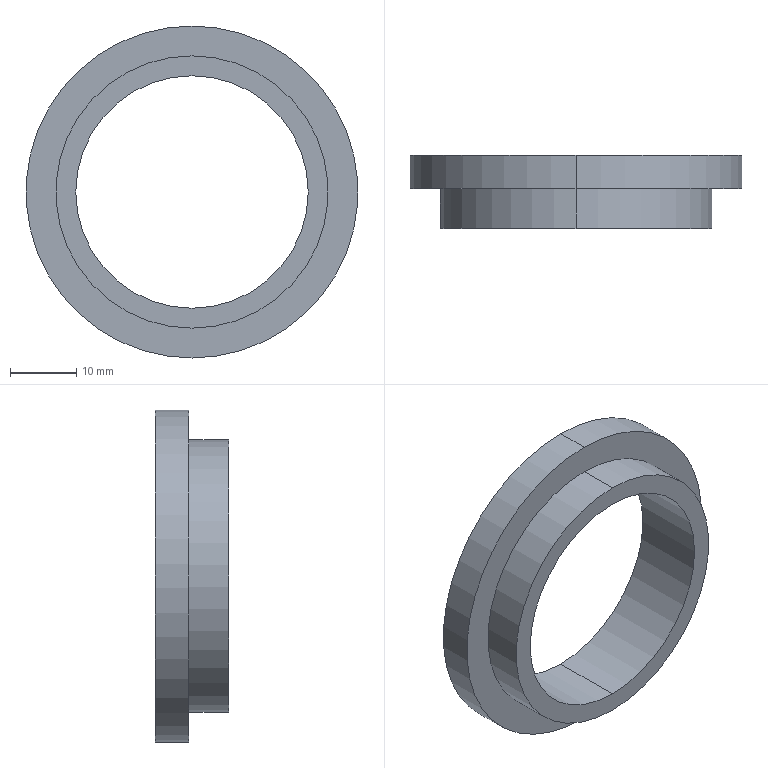Part | SolidWorks | features Revolution 1 | 1 solid | 9 faces | box 50 x 11 x 50 mm | volume 7156 mm3 | cylinder 6 | plane 3 | commonest cylinder face diameters 35 x2 41 x2 50 x2
STEP:
#1=CARTESIAN_POINT('',(0.,0.,20.5));
#2=VERTEX_POINT('',#1);
#3=CARTESIAN_POINT('',(0.,0.,-20.5));
#4=VERTEX_POINT('',#3);
#5=CARTESIAN_POINT('',(0.,0.,0.));
#6=DIRECTION('',(0.,1.,0.));
#7=DIRECTION('',(0.,0.,1.));
#8=AXIS2_PLACEMENT_3D('',#5,#6,#7);
#9=CIRCLE('',#8,20.5);
#10=EDGE_CURVE('',#2,#4,#9,.T.);
#11=ORIENTED_EDGE('',*,*,#10,.T.);
#12=CARTESIAN_POINT('',(0.,6.,-20.5));
#13=VERTEX_POINT('',#12);
#14=CARTESIAN_POINT('',(0.,46.272,-20.5));
#15=DIRECTION('',(0.,1.,0.));
#16=VECTOR('',#15,1000.);
#17=LINE('',#14,#16);
#18=EDGE_CURVE('',#4,#13,#17,.T.);
#19=ORIENTED_EDGE('',*,*,#18,.T.);
#20=CARTESIAN_POINT('',(0.,6.,20.5));
#21=VERTEX_POINT('',#20);
#22=CARTESIAN_POINT('',(0.,6.,0.));
#23=DIRECTION('',(0.,1.,0.));
#24=DIRECTION('',(0.,0.,1.));
#25=AXIS2_PLACEMENT_3D('',#22,#23,#24);
#26=CIRCLE('',#25,20.5);
#27=EDGE_CURVE('',#21,#13,#26,.T.);
#28=ORIENTED_EDGE('',*,*,#27,.F.);
#29=CARTESIAN_POINT('',(0.,46.272,20.5));
#30=DIRECTION('',(0.,1.,0.));
#31=VECTOR('',#30,1000.);
#32=LINE('',#29,#31);
#33=EDGE_CURVE('',#2,#21,#32,.T.);
#34=ORIENTED_EDGE('',*,*,#33,.F.);
#35=EDGE_LOOP('',(#11,#19,#28,#34));
#36=FACE_OUTER_BOUND('',#35,.T.);
#37=CARTESIAN_POINT('',(0.,46.272,0.));
#38=DIRECTION('',(0.,1.,0.));
#39=DIRECTION('',(0.,0.,1.));
#40=AXIS2_PLACEMENT_3D('',#37,#38,#39);
#41=CYLINDRICAL_SURFACE('',#40,20.5);
#42=ADVANCED_FACE('',(#36),#41,.T.);
#43=CARTESIAN_POINT('',(0.,6.,25.));
#44=VERTEX_POINT('',#43);
#45=CARTESIAN_POINT('',(0.,6.,-25.));
#46=VERTEX_POINT('',#45);
#47=CARTESIAN_POINT('',(0.,6.,0.));
#48=DIRECTION('',(0.,1.,0.));
#49=DIRECTION('',(0.,0.,1.));
#50=AXIS2_PLACEMENT_3D('',#47,#48,#49);
#51=CIRCLE('',#50,25.);
#52=EDGE_CURVE('',#44,#46,#51,.T.);
#53=ORIENTED_EDGE('',*,*,#52,.T.);
#54=CARTESIAN_POINT('',(0.,11.,-25.));
#55=VERTEX_POINT('',#54);
#56=CARTESIAN_POINT('',(0.,46.272,-25.));
#57=DIRECTION('',(0.,1.,0.));
#58=VECTOR('',#57,1000.);
#59=LINE('',#56,#58);
#60=EDGE_CURVE('',#46,#55,#59,.T.);
#61=ORIENTED_EDGE('',*,*,#60,.T.);
#62=CARTESIAN_POINT('',(0.,11.,25.));
#63=VERTEX_POINT('',#62);
#64=CARTESIAN_POINT('',(0.,11.,0.));
#65=DIRECTION('',(0.,1.,0.));
#66=DIRECTION('',(0.,0.,1.));
#67=AXIS2_PLACEMENT_3D('',#64,#65,#66);
#68=CIRCLE('',#67,25.);
#69=EDGE_CURVE('',#63,#55,#68,.T.);
#70=ORIENTED_EDGE('',*,*,#69,.F.);
#71=CARTESIAN_POINT('',(0.,46.272,25.));
#72=DIRECTION('',(0.,1.,0.));
#73=VECTOR('',#72,1000.);
#74=LINE('',#71,#73);
#75=EDGE_CURVE('',#44,#63,#74,.T.);
#76=ORIENTED_EDGE('',*,*,#75,.F.);
#77=EDGE_LOOP('',(#53,#61,#70,#76));
#78=FACE_OUTER_BOUND('',#77,.T.);
#79=CARTESIAN_POINT('',(0.,46.272,0.));
#80=DIRECTION('',(0.,1.,0.));
#81=DIRECTION('',(0.,0.,1.));
#82=AXIS2_PLACEMENT_3D('',#79,#80,#81);
#83=CYLINDRICAL_SURFACE('',#82,25.);
#84=ADVANCED_FACE('',(#78),#83,.T.);
#85=CARTESIAN_POINT('',(0.,0.,-17.5));
#86=VERTEX_POINT('',#85);
#87=CARTESIAN_POINT('',(0.,0.,17.5));
#88=VERTEX_POINT('',#87);
#89=CARTESIAN_POINT('',(0.,0.,0.));
#90=DIRECTION('',(0.,1.,0.));
#91=DIRECTION('',(0.,0.,1.));
#92=AXIS2_PLACEMENT_3D('',#89,#90,#91);
#93=CIRCLE('',#92,17.5);
#94=EDGE_CURVE('',#86,#88,#93,.T.);
#95=ORIENTED_EDGE('',*,*,#94,.F.);
#96=CARTESIAN_POINT('',(0.,11.,-17.5));
#97=VERTEX_POINT('',#96);
#98=CARTESIAN_POINT('',(0.,46.272,-17.5));
#99=DIRECTION('',(0.,1.,0.));
#100=VECTOR('',#99,1000.);
#101=LINE('',#98,#100);
#102=EDGE_CURVE('',#86,#97,#101,.T.);
#103=ORIENTED_EDGE('',*,*,#102,.T.);
#104=CARTESIAN_POINT('',(0.,11.,17.5));
#105=VERTEX_POINT('',#104);
#106=CARTESIAN_POINT('',(0.,11.,0.));
#107=DIRECTION('',(0.,1.,0.));
#108=DIRECTION('',(0.,0.,1.));
#109=AXIS2_PLACEMENT_3D('',#106,#107,#108);
#110=CIRCLE('',#109,17.5);
#111=EDGE_CURVE('',#97,#105,#110,.T.);
#112=ORIENTED_EDGE('',*,*,#111,.T.);
#113=CARTESIAN_POINT('',(0.,46.272,17.5));
#114=DIRECTION('',(0.,1.,0.));
#115=VECTOR('',#114,1000.);
#116=LINE('',#113,#115);
#117=EDGE_CURVE('',#88,#105,#116,.T.);
#118=ORIENTED_EDGE('',*,*,#117,.F.);
#119=EDGE_LOOP('',(#95,#103,#112,#118));
#120=FACE_OUTER_BOUND('',#119,.T.);
#121=CARTESIAN_POINT('',(0.,46.272,0.));
#122=DIRECTION('',(0.,1.,0.));
#123=DIRECTION('',(0.,0.,1.));
#124=AXIS2_PLACEMENT_3D('',#121,#122,#123);
#125=CYLINDRICAL_SURFACE('',#124,17.5);
#126=ADVANCED_FACE('',(#120),#125,.F.);
#127=ORIENTED_EDGE('',*,*,#10,.F.);
#128=CARTESIAN_POINT('',(0.,0.,0.));
#129=DIRECTION('',(0.,1.,0.));
#130=DIRECTION('',(0.,0.,1.));
#131=AXIS2_PLACEMENT_3D('',#128,#129,#130);
#132=CIRCLE('',#131,20.5);
#133=EDGE_CURVE('',#4,#2,#132,.T.);
#134=ORIENTED_EDGE('',*,*,#133,.F.);
#135=EDGE_LOOP('',(#127,#134));
#136=FACE_OUTER_BOUND('',#135,.T.);
#137=CARTESIAN_POINT('',(0.,0.,0.));
#138=DIRECTION('',(0.,1.,0.));
#139=DIRECTION('',(0.,0.,1.));
#140=AXIS2_PLACEMENT_3D('',#137,#138,#139);
#141=CIRCLE('',#140,17.5);
#142=EDGE_CURVE('',#88,#86,#141,.T.);
#143=ORIENTED_EDGE('',*,*,#142,.T.);
#144=ORIENTED_EDGE('',*,*,#94,.T.);
#145=EDGE_LOOP('',(#143,#144));
#146=FACE_BOUND('',#145,.T.);
#147=CARTESIAN_POINT('',(0.,0.,-20.5));
#148=DIRECTION('',(0.,1.,0.));
#149=DIRECTION('',(0.,0.,1.));
#150=AXIS2_PLACEMENT_3D('',#147,#148,#149);
#151=PLANE('',#150);
#152=ADVANCED_FACE('',(#136,#146),#151,.F.);
#153=ORIENTED_EDGE('',*,*,#102,.F.);
#154=ORIENTED_EDGE('',*,*,#142,.F.);
#155=ORIENTED_EDGE('',*,*,#117,.T.);
#156=CARTESIAN_POINT('',(0.,11.,0.));
#157=DIRECTION('',(0.,1.,0.));
#158=DIRECTION('',(0.,0.,1.));
#159=AXIS2_PLACEMENT_3D('',#156,#157,#158);
#160=CIRCLE('',#159,17.5);
#161=EDGE_CURVE('',#105,#97,#160,.T.);
#162=ORIENTED_EDGE('',*,*,#161,.T.);
#163=EDGE_LOOP('',(#153,#154,#155,#162));
#164=FACE_OUTER_BOUND('',#163,.T.);
#165=CARTESIAN_POINT('',(0.,46.272,0.));
#166=DIRECTION('',(0.,1.,0.));
#167=DIRECTION('',(0.,0.,1.));
#168=AXIS2_PLACEMENT_3D('',#165,#166,#167);
#169=CYLINDRICAL_SURFACE('',#168,17.5);
#170=ADVANCED_FACE('',(#164),#169,.F.);
#171=ORIENTED_EDGE('',*,*,#161,.F.);
#172=ORIENTED_EDGE('',*,*,#111,.F.);
#173=EDGE_LOOP('',(#171,#172));
#174=FACE_BOUND('',#173,.T.);
#175=ORIENTED_EDGE('',*,*,#69,.T.);
#176=CARTESIAN_POINT('',(0.,11.,0.));
#177=DIRECTION('',(0.,1.,0.));
#178=DIRECTION('',(0.,0.,1.));
#179=AXIS2_PLACEMENT_3D('',#176,#177,#178);
#180=CIRCLE('',#179,25.);
#181=EDGE_CURVE('',#55,#63,#180,.T.);
#182=ORIENTED_EDGE('',*,*,#181,.T.);
#183=EDGE_LOOP('',(#175,#182));
#184=FACE_OUTER_BOUND('',#183,.T.);
#185=CARTESIAN_POINT('',(0.,11.,-17.5));
#186=DIRECTION('',(0.,-1.,0.));
#187=DIRECTION('',(0.,0.,-1.));
#188=AXIS2_PLACEMENT_3D('',#185,#186,#187);
#189=PLANE('',#188);
#190=ADVANCED_FACE('',(#174,#184),#189,.F.);
#191=ORIENTED_EDGE('',*,*,#60,.F.);
#192=CARTESIAN_POINT('',(0.,6.,0.));
#193=DIRECTION('',(0.,1.,0.));
#194=DIRECTION('',(0.,0.,1.));
#195=AXIS2_PLACEMENT_3D('',#192,#193,#194);
#196=CIRCLE('',#195,25.);
#197=EDGE_CURVE('',#46,#44,#196,.T.);
#198=ORIENTED_EDGE('',*,*,#197,.T.);
#199=ORIENTED_EDGE('',*,*,#75,.T.);
#200=ORIENTED_EDGE('',*,*,#181,.F.);
#201=EDGE_LOOP('',(#191,#198,#199,#200));
#202=FACE_OUTER_BOUND('',#201,.T.);
#203=CARTESIAN_POINT('',(0.,46.272,0.));
#204=DIRECTION('',(0.,1.,0.));
#205=DIRECTION('',(0.,0.,1.));
#206=AXIS2_PLACEMENT_3D('',#203,#204,#205);
#207=CYLINDRICAL_SURFACE('',#206,25.);
#208=ADVANCED_FACE('',(#202),#207,.T.);
#209=ORIENTED_EDGE('',*,*,#52,.F.);
#210=ORIENTED_EDGE('',*,*,#197,.F.);
#211=EDGE_LOOP('',(#209,#210));
#212=FACE_OUTER_BOUND('',#211,.T.);
#213=ORIENTED_EDGE('',*,*,#27,.T.);
#214=CARTESIAN_POINT('',(0.,6.,0.));
#215=DIRECTION('',(0.,1.,0.));
#216=DIRECTION('',(0.,0.,1.));
#217=AXIS2_PLACEMENT_3D('',#214,#215,#216);
#218=CIRCLE('',#217,20.5);
#219=EDGE_CURVE('',#13,#21,#218,.T.);
#220=ORIENTED_EDGE('',*,*,#219,.T.);
#221=EDGE_LOOP('',(#213,#220));
#222=FACE_BOUND('',#221,.T.);
#223=CARTESIAN_POINT('',(0.,6.,-25.));
#224=DIRECTION('',(0.,1.,0.));
#225=DIRECTION('',(0.,0.,1.));
#226=AXIS2_PLACEMENT_3D('',#223,#224,#225);
#227=PLANE('',#226);
#228=ADVANCED_FACE('',(#212,#222),#227,.F.);
#229=ORIENTED_EDGE('',*,*,#18,.F.);
#230=ORIENTED_EDGE('',*,*,#133,.T.);
#231=ORIENTED_EDGE('',*,*,#33,.T.);
#232=ORIENTED_EDGE('',*,*,#219,.F.);
#233=EDGE_LOOP('',(#229,#230,#231,#232));
#234=FACE_OUTER_BOUND('',#233,.T.);
#235=CARTESIAN_POINT('',(0.,46.272,0.));
#236=DIRECTION('',(0.,1.,0.));
#237=DIRECTION('',(0.,0.,1.));
#238=AXIS2_PLACEMENT_3D('',#235,#236,#237);
#239=CYLINDRICAL_SURFACE('',#238,20.5);
#240=ADVANCED_FACE('',(#234),#239,.T.);
#241=CLOSED_SHELL('',(#42,#84,#126,#152,#170,#190,#208,#228,#240));
#242=MANIFOLD_SOLID_BREP('',#241);
#243=CARTESIAN_POINT('',(0.,0.,0.));
#244=DIRECTION('',(0.,0.,1.));
#245=DIRECTION('',(1.,0.,0.));
#246=AXIS2_PLACEMENT_3D('',#243,#244,#245);
#247=(LENGTH_UNIT()NAMED_UNIT(*)SI_UNIT(.MILLI.,.METRE.));
#248=UNCERTAINTY_MEASURE_WITH_UNIT(LENGTH_MEASURE(0.00001),#247,'','');
#249=(NAMED_UNIT(*)PLANE_ANGLE_UNIT()SI_UNIT($,.RADIAN.));
#250=(NAMED_UNIT(*)SI_UNIT($,.STERADIAN.)SOLID_ANGLE_UNIT());
#251=(GEOMETRIC_REPRESENTATION_CONTEXT(3)GLOBAL_UNCERTAINTY_ASSIGNED_CONTEXT((#248))GLOBAL_UNIT_ASSIGNED_CONTEXT((#247,#249,#250))REPRESENTATION_CONTEXT('',''));
#252=ADVANCED_BREP_SHAPE_REPRESENTATION('',(#242,#246),#251);